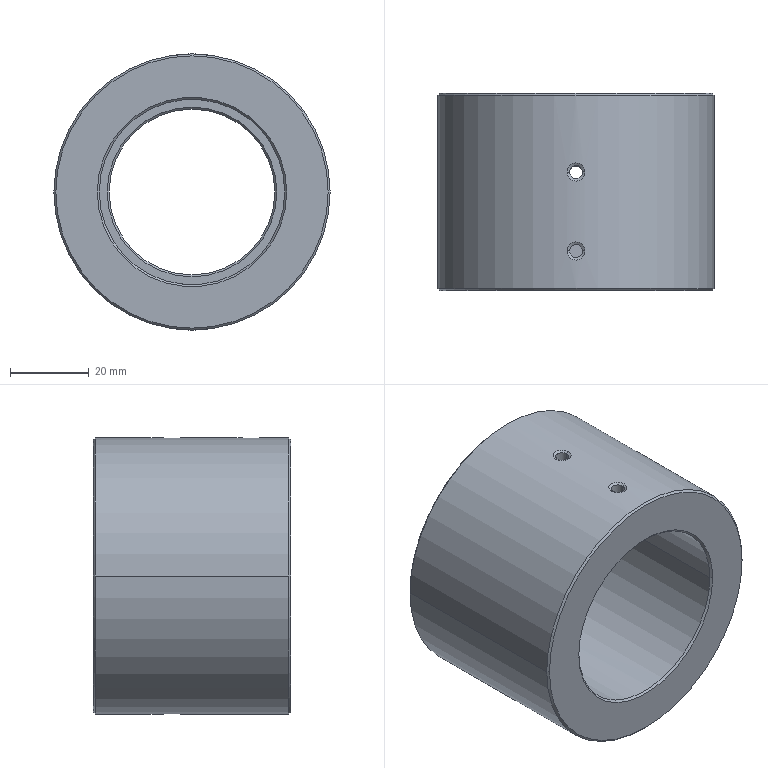Part | NX | 1 solid | 63 faces | box 70 x 50 x 70 mm | volume 106582 mm3 | cylinder 28 | cone 26 | spline 6 | plane 3 | commonest cylinder face diameters 3.3 x22 42 x2 47 x2 70 x2